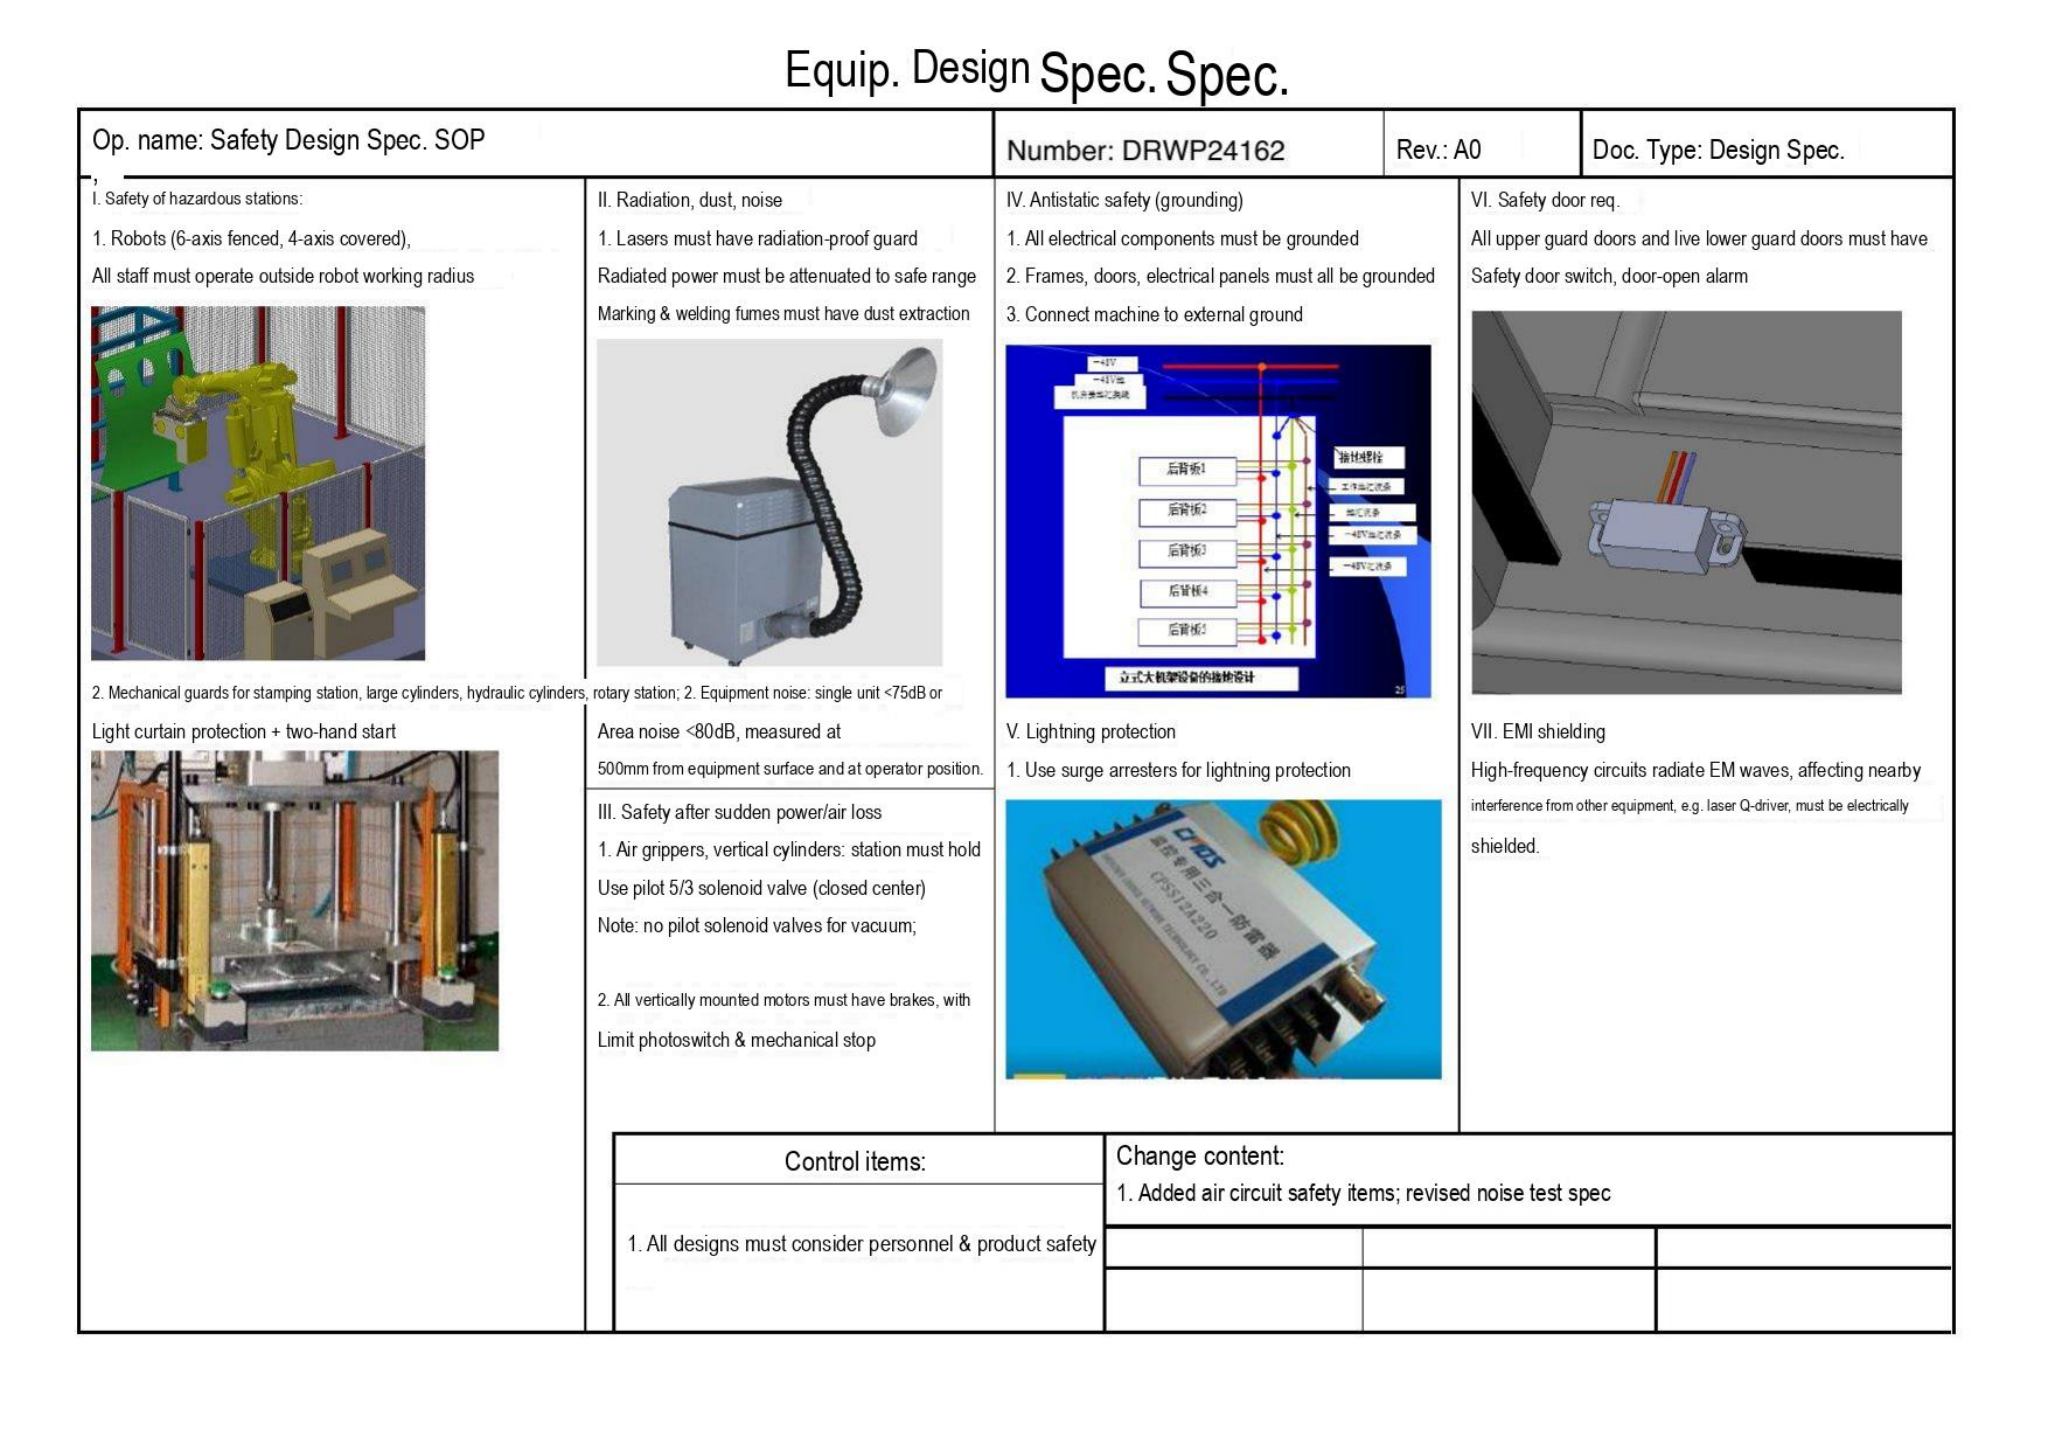# Equip. Design Spec. Spec.

| Op. name: Safety Design Spec. SOP | Number: DRWP24162 | Rev.: A0 | Doc. Type: Design Spec. |
|---|---|---|---|

I. Safety of hazardous stations:

1. Robots (6-axis fenced, 4-axis covered),

All staff must operate outside robot working radius

2. Mechanical guards for stamping station, large cylinders, hydraulic cylinders, rotary station;

Light curtain protection + two-hand start

II. Radiation, dust, noise

1. Lasers must have radiation-proof guard

Radiated power must be attenuated to safe range

Marking & welding fumes must have dust extraction

2. Equipment noise: single unit <75dB or

Area noise <80dB, measured at

500mm from equipment surface and at operator position.

III. Safety after sudden power/air loss

1. Air grippers, vertical cylinders: station must hold

Use pilot 5/3 solenoid valve (closed center)

Note: no pilot solenoid valves for vacuum;

2. All vertically mounted motors must have brakes, with

Limit photoswitch & mechanical stop

IV. Antistatic safety (grounding)

1. All electrical components must be grounded

2. Frames, doors, electrical panels must all be grounded

3. Connect machine to external ground

-48V

后背板1

后背板2

后背板3

后背板4

后背板5

立式大机架设备的接地设计

V. Lightning protection

1. Use surge arresters for lightning protection

CPSS12A220

VI. Safety door req.

All upper guard doors and live lower guard doors must have

Safety door switch, door-open alarm

VII. EMI shielding

High-frequency circuits radiate EM waves, affecting nearby

interference from other equipment, e.g. laser Q-driver, must be electrically

shielded.

| Control items: | Change content: 1. Added air circuit safety items; revised noise test spec | | |
|---|---|---|---|
| 1. All designs must consider personnel & product safety | | | |
| | | | |
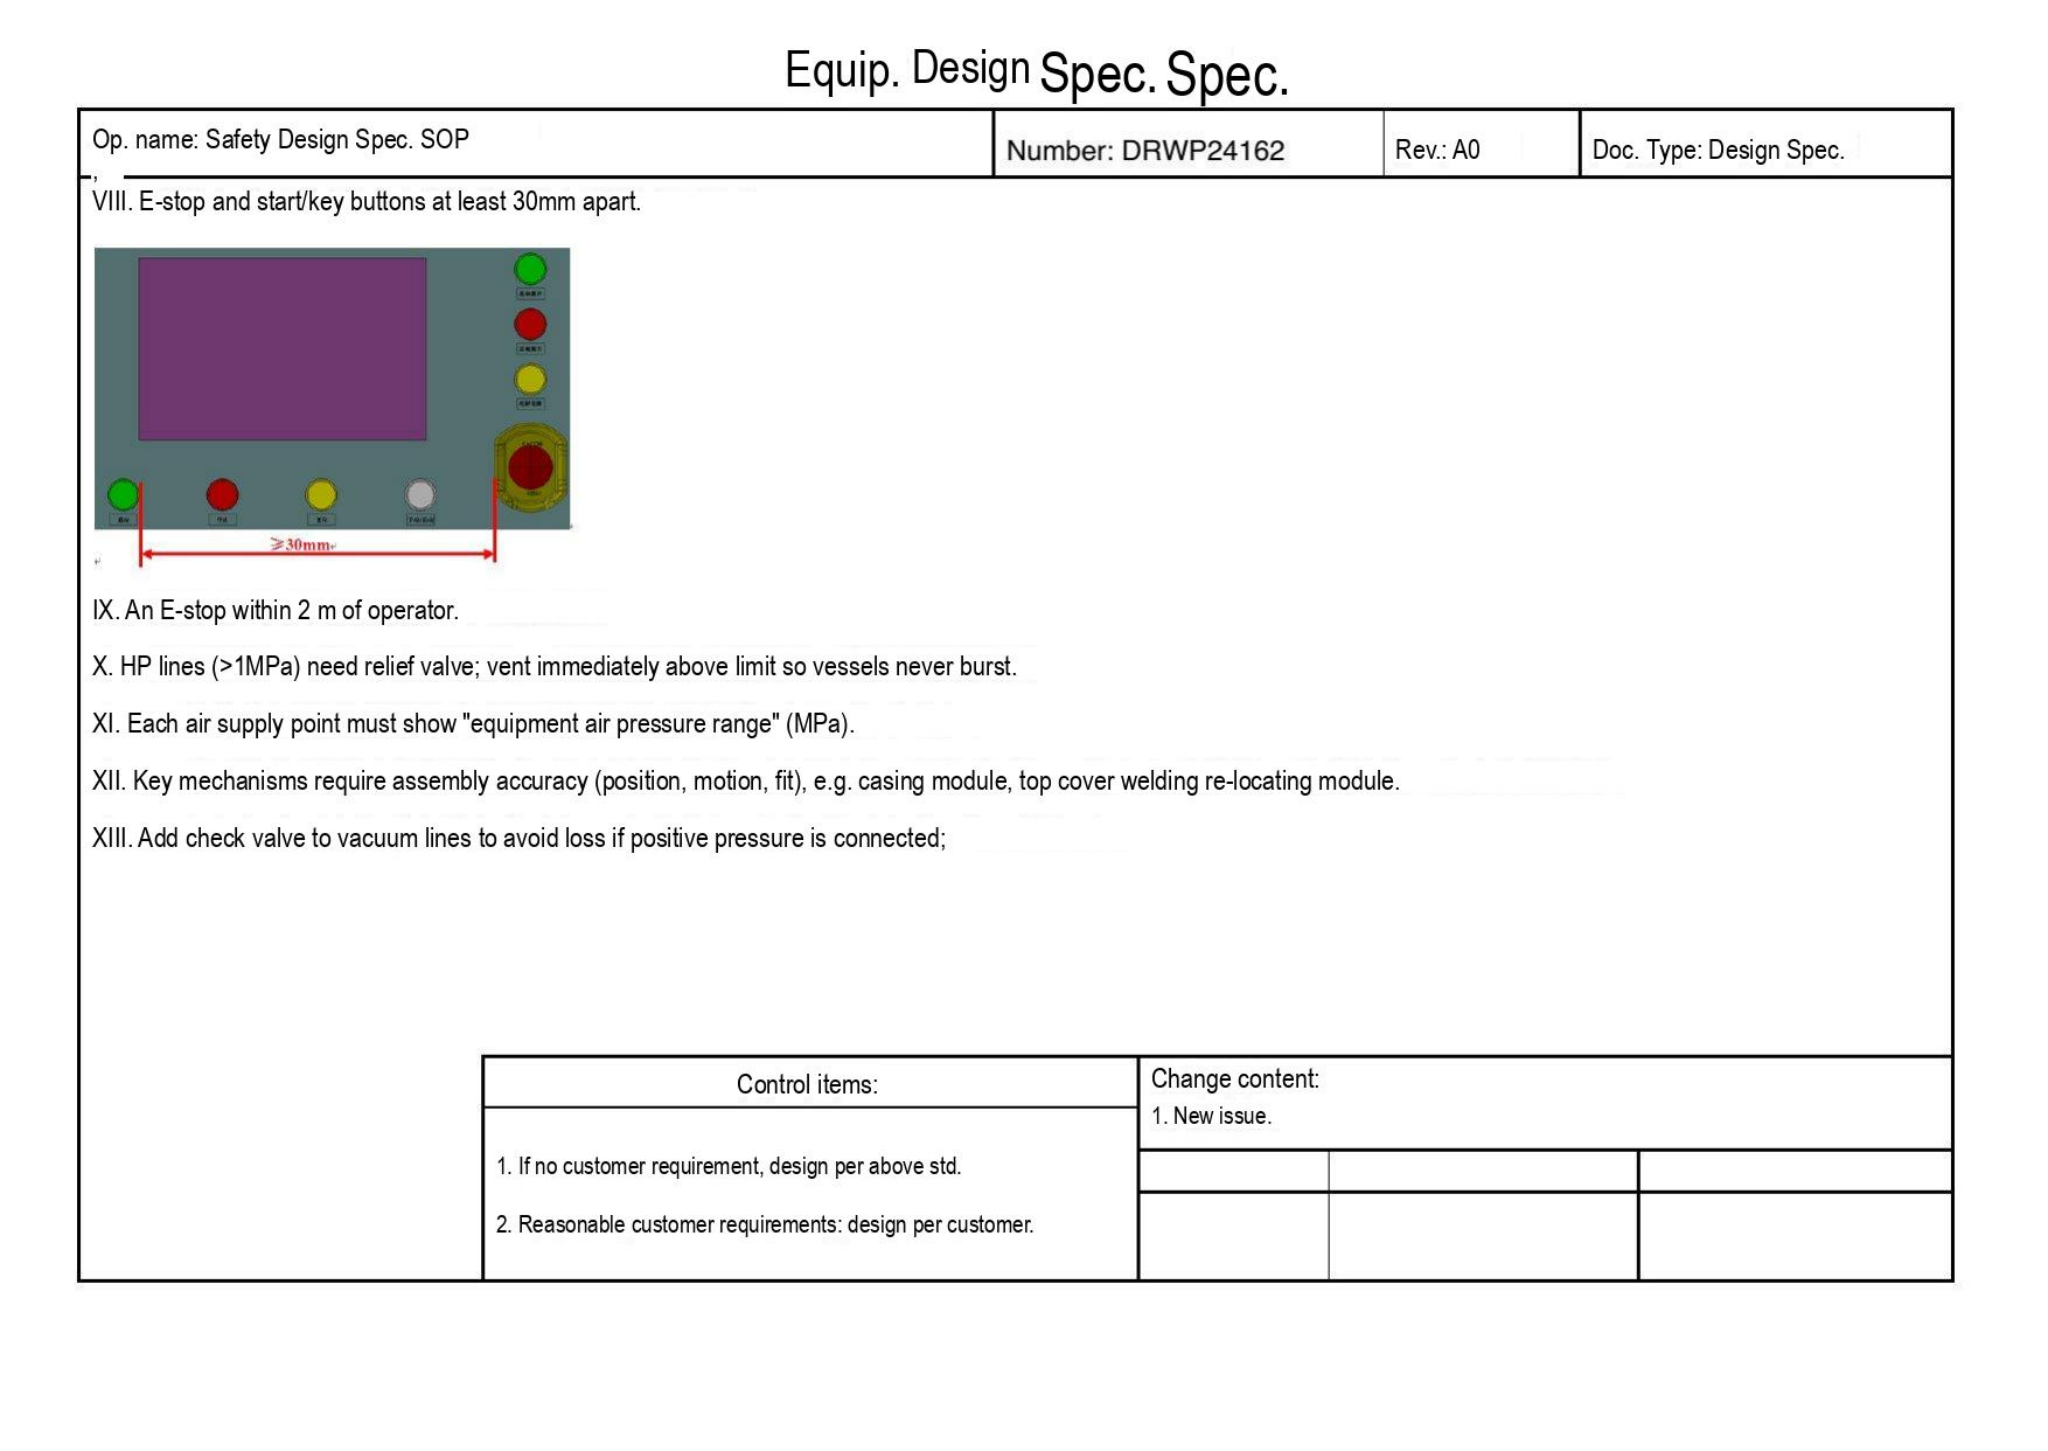Equip. Design Spec. Spec.

| Op. name: Safety Design Spec. SOP | Number: DRWP24162 | Rev.: A0 | Doc. Type: Design Spec. |
|---|---|---|---|

VIII. E-stop and start/key buttons at least 30mm apart.

≥30mm

IX. An E-stop within 2 m of operator.

X. HP lines (>1MPa) need relief valve; vent immediately above limit so vessels never burst.

XI. Each air supply point must show "equipment air pressure range" (MPa).

XII. Key mechanisms require assembly accuracy (position, motion, fit), e.g. casing module, top cover welding re-locating module.

XIII. Add check valve to vacuum lines to avoid loss if positive pressure is connected;

| Control items: | Change content: 1. New issue. | | |
|---|---|---|---|
| 1. If no customer requirement, design per above std. 2. Reasonable customer requirements: design per customer. | | | |
| | | | |